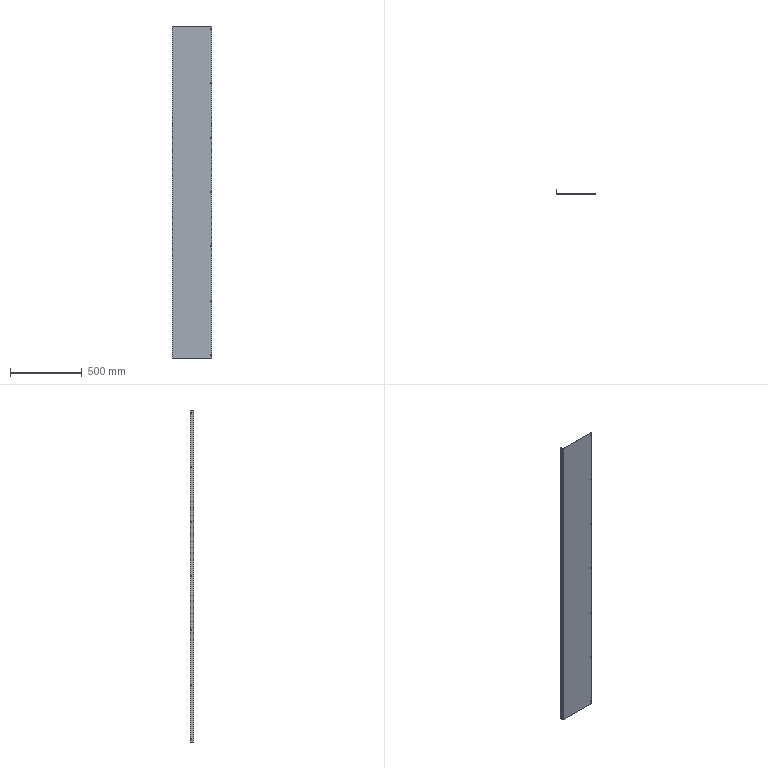Part | 1 solid | 70 faces | box 279 x 24 x 2316 mm | volume 698088 mm3 | plane 40 | cylinder 30 | commonest cylinder face diameters 6 x28 0.4 x1 2.4 x1